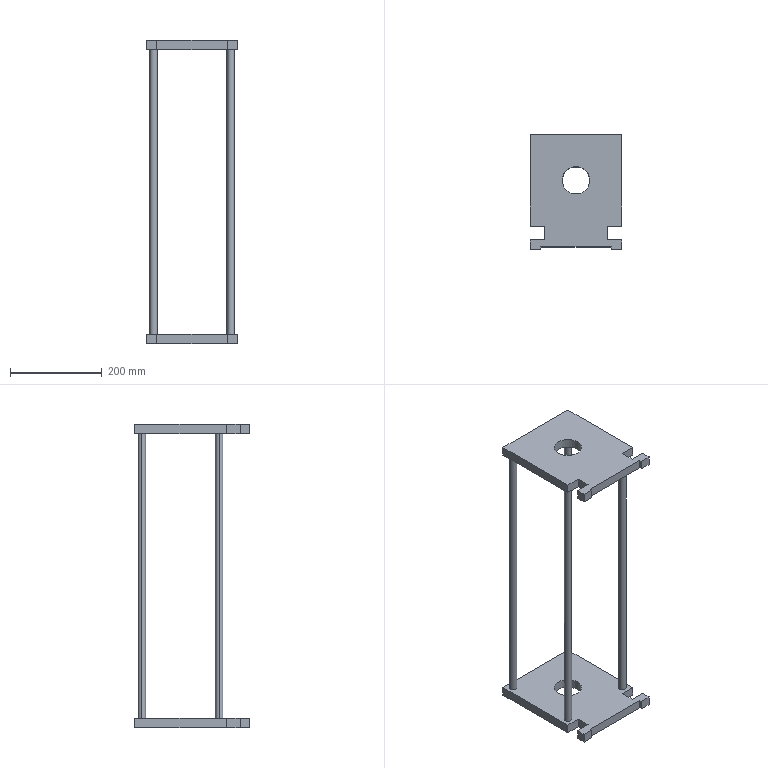Part | SolidWorks | features ICE 2, Extrusion 1 | 1 solid | 48 faces | box 200 x 250 x 660 mm | volume 2278181 mm3 | plane 36 | cylinder 12 | commonest cylinder face diameters 16 x8 60 x4
STEP:
#1=CARTESIAN_POINT('',(-30.,145.,660.));
#2=VERTEX_POINT('',#1);
#3=CARTESIAN_POINT('',(30.,145.,660.));
#4=VERTEX_POINT('',#3);
#5=CARTESIAN_POINT('',(0.,145.,660.));
#6=DIRECTION('',(0.,0.,1.));
#7=DIRECTION('',(1.,0.,0.));
#8=AXIS2_PLACEMENT_3D('',#5,#6,#7);
#9=CIRCLE('',#8,30.);
#10=EDGE_CURVE('',#2,#4,#9,.T.);
#11=ORIENTED_EDGE('',*,*,#10,.T.);
#12=CARTESIAN_POINT('',(30.,145.,640.));
#13=VERTEX_POINT('',#12);
#14=CARTESIAN_POINT('',(30.,145.,660.));
#15=DIRECTION('',(0.,0.,-1.));
#16=VECTOR('',#15,1000.);
#17=LINE('',#14,#16);
#18=EDGE_CURVE('',#4,#13,#17,.T.);
#19=ORIENTED_EDGE('',*,*,#18,.T.);
#20=CARTESIAN_POINT('',(-30.,145.,640.));
#21=VERTEX_POINT('',#20);
#22=CARTESIAN_POINT('',(0.,145.,640.));
#23=DIRECTION('',(0.,0.,1.));
#24=DIRECTION('',(1.,0.,0.));
#25=AXIS2_PLACEMENT_3D('',#22,#23,#24);
#26=CIRCLE('',#25,30.);
#27=EDGE_CURVE('',#21,#13,#26,.T.);
#28=ORIENTED_EDGE('',*,*,#27,.F.);
#29=CARTESIAN_POINT('',(-30.,145.,660.));
#30=DIRECTION('',(0.,0.,-1.));
#31=VECTOR('',#30,1000.);
#32=LINE('',#29,#31);
#33=EDGE_CURVE('',#2,#21,#32,.T.);
#34=ORIENTED_EDGE('',*,*,#33,.F.);
#35=EDGE_LOOP('',(#11,#19,#28,#34));
#36=FACE_OUTER_BOUND('',#35,.T.);
#37=CARTESIAN_POINT('',(0.,145.,660.));
#38=DIRECTION('',(0.,0.,-1.));
#39=DIRECTION('',(-1.,0.,0.));
#40=AXIS2_PLACEMENT_3D('',#37,#38,#39);
#41=CYLINDRICAL_SURFACE('',#40,30.);
#42=ADVANCED_FACE('',(#36),#41,.F.);
#43=CARTESIAN_POINT('',(-76.,61.,640.));
#44=VERTEX_POINT('',#43);
#45=CARTESIAN_POINT('',(-92.,61.,640.));
#46=VERTEX_POINT('',#45);
#47=CARTESIAN_POINT('',(-84.,61.,640.));
#48=DIRECTION('',(0.,0.,1.));
#49=DIRECTION('',(1.,0.,0.));
#50=AXIS2_PLACEMENT_3D('',#47,#48,#49);
#51=CIRCLE('',#50,8.);
#52=EDGE_CURVE('',#44,#46,#51,.T.);
#53=ORIENTED_EDGE('',*,*,#52,.F.);
#54=CARTESIAN_POINT('',(-76.,61.,20.));
#55=VERTEX_POINT('',#54);
#56=CARTESIAN_POINT('',(-76.,61.,640.));
#57=DIRECTION('',(0.,0.,-1.));
#58=VECTOR('',#57,1000.);
#59=LINE('',#56,#58);
#60=EDGE_CURVE('',#44,#55,#59,.T.);
#61=ORIENTED_EDGE('',*,*,#60,.T.);
#62=CARTESIAN_POINT('',(-92.,61.,20.));
#63=VERTEX_POINT('',#62);
#64=CARTESIAN_POINT('',(-84.,61.,20.));
#65=DIRECTION('',(0.,0.,1.));
#66=DIRECTION('',(-1.,0.,0.));
#67=AXIS2_PLACEMENT_3D('',#64,#65,#66);
#68=CIRCLE('',#67,8.);
#69=EDGE_CURVE('',#55,#63,#68,.T.);
#70=ORIENTED_EDGE('',*,*,#69,.T.);
#71=CARTESIAN_POINT('',(-92.,61.,640.));
#72=DIRECTION('',(0.,0.,-1.));
#73=VECTOR('',#72,1000.);
#74=LINE('',#71,#73);
#75=EDGE_CURVE('',#46,#63,#74,.T.);
#76=ORIENTED_EDGE('',*,*,#75,.F.);
#77=EDGE_LOOP('',(#53,#61,#70,#76));
#78=FACE_OUTER_BOUND('',#77,.T.);
#79=CARTESIAN_POINT('',(-84.,61.,640.));
#80=DIRECTION('',(0.,0.,-1.));
#81=DIRECTION('',(-1.,0.,0.));
#82=AXIS2_PLACEMENT_3D('',#79,#80,#81);
#83=CYLINDRICAL_SURFACE('',#82,8.);
#84=ADVANCED_FACE('',(#78),#83,.T.);
#85=CARTESIAN_POINT('',(92.,61.,640.));
#86=VERTEX_POINT('',#85);
#87=CARTESIAN_POINT('',(76.,61.,640.));
#88=VERTEX_POINT('',#87);
#89=CARTESIAN_POINT('',(84.,61.,640.));
#90=DIRECTION('',(0.,0.,1.));
#91=DIRECTION('',(1.,0.,0.));
#92=AXIS2_PLACEMENT_3D('',#89,#90,#91);
#93=CIRCLE('',#92,8.);
#94=EDGE_CURVE('',#86,#88,#93,.T.);
#95=ORIENTED_EDGE('',*,*,#94,.F.);
#96=CARTESIAN_POINT('',(92.,61.,20.));
#97=VERTEX_POINT('',#96);
#98=CARTESIAN_POINT('',(92.,61.,640.));
#99=DIRECTION('',(0.,0.,-1.));
#100=VECTOR('',#99,1000.);
#101=LINE('',#98,#100);
#102=EDGE_CURVE('',#86,#97,#101,.T.);
#103=ORIENTED_EDGE('',*,*,#102,.T.);
#104=CARTESIAN_POINT('',(76.,61.,20.));
#105=VERTEX_POINT('',#104);
#106=CARTESIAN_POINT('',(84.,61.,20.));
#107=DIRECTION('',(0.,0.,1.));
#108=DIRECTION('',(-1.,0.,0.));
#109=AXIS2_PLACEMENT_3D('',#106,#107,#108);
#110=CIRCLE('',#109,8.);
#111=EDGE_CURVE('',#97,#105,#110,.T.);
#112=ORIENTED_EDGE('',*,*,#111,.T.);
#113=CARTESIAN_POINT('',(76.,61.,640.));
#114=DIRECTION('',(0.,0.,-1.));
#115=VECTOR('',#114,1000.);
#116=LINE('',#113,#115);
#117=EDGE_CURVE('',#88,#105,#116,.T.);
#118=ORIENTED_EDGE('',*,*,#117,.F.);
#119=EDGE_LOOP('',(#95,#103,#112,#118));
#120=FACE_OUTER_BOUND('',#119,.T.);
#121=CARTESIAN_POINT('',(84.,61.,640.));
#122=DIRECTION('',(0.,0.,-1.));
#123=DIRECTION('',(-1.,0.,0.));
#124=AXIS2_PLACEMENT_3D('',#121,#122,#123);
#125=CYLINDRICAL_SURFACE('',#124,8.);
#126=ADVANCED_FACE('',(#120),#125,.T.);
#127=CARTESIAN_POINT('',(92.,229.,640.));
#128=VERTEX_POINT('',#127);
#129=CARTESIAN_POINT('',(76.,229.,640.));
#130=VERTEX_POINT('',#129);
#131=CARTESIAN_POINT('',(84.,229.,640.));
#132=DIRECTION('',(0.,0.,1.));
#133=DIRECTION('',(1.,0.,0.));
#134=AXIS2_PLACEMENT_3D('',#131,#132,#133);
#135=CIRCLE('',#134,8.);
#136=EDGE_CURVE('',#128,#130,#135,.T.);
#137=ORIENTED_EDGE('',*,*,#136,.F.);
#138=CARTESIAN_POINT('',(92.,229.,20.));
#139=VERTEX_POINT('',#138);
#140=CARTESIAN_POINT('',(92.,229.,640.));
#141=DIRECTION('',(0.,0.,-1.));
#142=VECTOR('',#141,1000.);
#143=LINE('',#140,#142);
#144=EDGE_CURVE('',#128,#139,#143,.T.);
#145=ORIENTED_EDGE('',*,*,#144,.T.);
#146=CARTESIAN_POINT('',(76.,229.,20.));
#147=VERTEX_POINT('',#146);
#148=CARTESIAN_POINT('',(84.,229.,20.));
#149=DIRECTION('',(0.,0.,1.));
#150=DIRECTION('',(-1.,0.,0.));
#151=AXIS2_PLACEMENT_3D('',#148,#149,#150);
#152=CIRCLE('',#151,8.);
#153=EDGE_CURVE('',#139,#147,#152,.T.);
#154=ORIENTED_EDGE('',*,*,#153,.T.);
#155=CARTESIAN_POINT('',(76.,229.,640.));
#156=DIRECTION('',(0.,0.,-1.));
#157=VECTOR('',#156,1000.);
#158=LINE('',#155,#157);
#159=EDGE_CURVE('',#130,#147,#158,.T.);
#160=ORIENTED_EDGE('',*,*,#159,.F.);
#161=EDGE_LOOP('',(#137,#145,#154,#160));
#162=FACE_OUTER_BOUND('',#161,.T.);
#163=CARTESIAN_POINT('',(84.,229.,640.));
#164=DIRECTION('',(0.,0.,-1.));
#165=DIRECTION('',(-1.,0.,0.));
#166=AXIS2_PLACEMENT_3D('',#163,#164,#165);
#167=CYLINDRICAL_SURFACE('',#166,8.);
#168=ADVANCED_FACE('',(#162),#167,.T.);
#169=CARTESIAN_POINT('',(-76.,229.,640.));
#170=VERTEX_POINT('',#169);
#171=CARTESIAN_POINT('',(-92.,229.,640.));
#172=VERTEX_POINT('',#171);
#173=CARTESIAN_POINT('',(-84.,229.,640.));
#174=DIRECTION('',(0.,0.,1.));
#175=DIRECTION('',(1.,0.,0.));
#176=AXIS2_PLACEMENT_3D('',#173,#174,#175);
#177=CIRCLE('',#176,8.);
#178=EDGE_CURVE('',#170,#172,#177,.T.);
#179=ORIENTED_EDGE('',*,*,#178,.F.);
#180=CARTESIAN_POINT('',(-76.,229.,20.));
#181=VERTEX_POINT('',#180);
#182=CARTESIAN_POINT('',(-76.,229.,640.));
#183=DIRECTION('',(0.,0.,-1.));
#184=VECTOR('',#183,1000.);
#185=LINE('',#182,#184);
#186=EDGE_CURVE('',#170,#181,#185,.T.);
#187=ORIENTED_EDGE('',*,*,#186,.T.);
#188=CARTESIAN_POINT('',(-92.,229.,20.));
#189=VERTEX_POINT('',#188);
#190=CARTESIAN_POINT('',(-84.,229.,20.));
#191=DIRECTION('',(0.,0.,1.));
#192=DIRECTION('',(-1.,0.,0.));
#193=AXIS2_PLACEMENT_3D('',#190,#191,#192);
#194=CIRCLE('',#193,8.);
#195=EDGE_CURVE('',#181,#189,#194,.T.);
#196=ORIENTED_EDGE('',*,*,#195,.T.);
#197=CARTESIAN_POINT('',(-92.,229.,640.));
#198=DIRECTION('',(0.,0.,-1.));
#199=VECTOR('',#198,1000.);
#200=LINE('',#197,#199);
#201=EDGE_CURVE('',#172,#189,#200,.T.);
#202=ORIENTED_EDGE('',*,*,#201,.F.);
#203=EDGE_LOOP('',(#179,#187,#196,#202));
#204=FACE_OUTER_BOUND('',#203,.T.);
#205=CARTESIAN_POINT('',(-84.,229.,640.));
#206=DIRECTION('',(0.,0.,-1.));
#207=DIRECTION('',(-1.,0.,0.));
#208=AXIS2_PLACEMENT_3D('',#205,#206,#207);
#209=CYLINDRICAL_SURFACE('',#208,8.);
#210=ADVANCED_FACE('',(#204),#209,.T.);
#211=CARTESIAN_POINT('',(-30.,145.,20.));
#212=VERTEX_POINT('',#211);
#213=CARTESIAN_POINT('',(30.,145.,20.));
#214=VERTEX_POINT('',#213);
#215=CARTESIAN_POINT('',(0.,145.,20.));
#216=DIRECTION('',(0.,0.,1.));
#217=DIRECTION('',(1.,0.,0.));
#218=AXIS2_PLACEMENT_3D('',#215,#216,#217);
#219=CIRCLE('',#218,30.);
#220=EDGE_CURVE('',#212,#214,#219,.T.);
#221=ORIENTED_EDGE('',*,*,#220,.T.);
#222=CARTESIAN_POINT('',(30.,145.,0.));
#223=VERTEX_POINT('',#222);
#224=CARTESIAN_POINT('',(30.,145.,20.));
#225=DIRECTION('',(0.,0.,-1.));
#226=VECTOR('',#225,1000.);
#227=LINE('',#224,#226);
#228=EDGE_CURVE('',#214,#223,#227,.T.);
#229=ORIENTED_EDGE('',*,*,#228,.T.);
#230=CARTESIAN_POINT('',(-30.,145.,0.));
#231=VERTEX_POINT('',#230);
#232=CARTESIAN_POINT('',(0.,145.,0.));
#233=DIRECTION('',(0.,0.,1.));
#234=DIRECTION('',(1.,0.,0.));
#235=AXIS2_PLACEMENT_3D('',#232,#233,#234);
#236=CIRCLE('',#235,30.);
#237=EDGE_CURVE('',#231,#223,#236,.T.);
#238=ORIENTED_EDGE('',*,*,#237,.F.);
#239=CARTESIAN_POINT('',(-30.,145.,20.));
#240=DIRECTION('',(0.,0.,-1.));
#241=VECTOR('',#240,1000.);
#242=LINE('',#239,#241);
#243=EDGE_CURVE('',#212,#231,#242,.T.);
#244=ORIENTED_EDGE('',*,*,#243,.F.);
#245=EDGE_LOOP('',(#221,#229,#238,#244));
#246=FACE_OUTER_BOUND('',#245,.T.);
#247=CARTESIAN_POINT('',(0.,145.,20.));
#248=DIRECTION('',(0.,0.,-1.));
#249=DIRECTION('',(-1.,0.,0.));
#250=AXIS2_PLACEMENT_3D('',#247,#248,#249);
#251=CYLINDRICAL_SURFACE('',#250,30.);
#252=ADVANCED_FACE('',(#246),#251,.F.);
#253=CARTESIAN_POINT('',(-84.,61.,20.));
#254=DIRECTION('',(0.,0.,1.));
#255=DIRECTION('',(-1.,0.,0.));
#256=AXIS2_PLACEMENT_3D('',#253,#254,#255);
#257=CIRCLE('',#256,8.);
#258=EDGE_CURVE('',#63,#55,#257,.T.);
#259=ORIENTED_EDGE('',*,*,#258,.F.);
#260=ORIENTED_EDGE('',*,*,#69,.F.);
#261=EDGE_LOOP('',(#259,#260));
#262=FACE_BOUND('',#261,.T.);
#263=CARTESIAN_POINT('',(84.,61.,20.));
#264=DIRECTION('',(0.,0.,1.));
#265=DIRECTION('',(-1.,0.,0.));
#266=AXIS2_PLACEMENT_3D('',#263,#264,#265);
#267=CIRCLE('',#266,8.);
#268=EDGE_CURVE('',#105,#97,#267,.T.);
#269=ORIENTED_EDGE('',*,*,#268,.F.);
#270=ORIENTED_EDGE('',*,*,#111,.F.);
#271=EDGE_LOOP('',(#269,#270));
#272=FACE_BOUND('',#271,.T.);
#273=CARTESIAN_POINT('',(84.,229.,20.));
#274=DIRECTION('',(0.,0.,1.));
#275=DIRECTION('',(-1.,0.,0.));
#276=AXIS2_PLACEMENT_3D('',#273,#274,#275);
#277=CIRCLE('',#276,8.);
#278=EDGE_CURVE('',#147,#139,#277,.T.);
#279=ORIENTED_EDGE('',*,*,#278,.F.);
#280=ORIENTED_EDGE('',*,*,#153,.F.);
#281=EDGE_LOOP('',(#279,#280));
#282=FACE_BOUND('',#281,.T.);
#283=CARTESIAN_POINT('',(-84.,229.,20.));
#284=DIRECTION('',(0.,0.,1.));
#285=DIRECTION('',(-1.,0.,0.));
#286=AXIS2_PLACEMENT_3D('',#283,#284,#285);
#287=CIRCLE('',#286,8.);
#288=EDGE_CURVE('',#189,#181,#287,.T.);
#289=ORIENTED_EDGE('',*,*,#288,.F.);
#290=ORIENTED_EDGE('',*,*,#195,.F.);
#291=EDGE_LOOP('',(#289,#290));
#292=FACE_BOUND('',#291,.T.);
#293=CARTESIAN_POINT('',(-76.389,-5.,20.));
#294=VERTEX_POINT('',#293);
#295=CARTESIAN_POINT('',(-76.389,0.,20.));
#296=VERTEX_POINT('',#295);
#297=CARTESIAN_POINT('',(-76.389,0.,20.));
#298=DIRECTION('',(0.,1.,0.));
#299=VECTOR('',#298,1000.);
#300=LINE('',#297,#299);
#301=EDGE_CURVE('',#294,#296,#300,.T.);
#302=ORIENTED_EDGE('',*,*,#301,.T.);
#303=CARTESIAN_POINT('',(76.389,0.,20.));
#304=VERTEX_POINT('',#303);
#305=CARTESIAN_POINT('',(76.389,0.,20.));
#306=DIRECTION('',(1.,0.,0.));
#307=VECTOR('',#306,1000.);
#308=LINE('',#305,#307);
#309=EDGE_CURVE('',#296,#304,#308,.T.);
#310=ORIENTED_EDGE('',*,*,#309,.T.);
#311=CARTESIAN_POINT('',(76.389,-5.,20.));
#312=VERTEX_POINT('',#311);
#313=CARTESIAN_POINT('',(76.389,0.,20.));
#314=DIRECTION('',(0.,-1.,0.));
#315=VECTOR('',#314,1000.);
#316=LINE('',#313,#315);
#317=EDGE_CURVE('',#304,#312,#316,.T.);
#318=ORIENTED_EDGE('',*,*,#317,.T.);
#319=CARTESIAN_POINT('',(100.,-5.,20.));
#320=VERTEX_POINT('',#319);
#321=CARTESIAN_POINT('',(76.389,-5.,20.));
#322=DIRECTION('',(1.,0.,0.));
#323=VECTOR('',#322,1000.);
#324=LINE('',#321,#323);
#325=EDGE_CURVE('',#312,#320,#324,.T.);
#326=ORIENTED_EDGE('',*,*,#325,.T.);
#327=CARTESIAN_POINT('',(100.,15.,20.));
#328=VERTEX_POINT('',#327);
#329=CARTESIAN_POINT('',(100.,-5.,20.));
#330=DIRECTION('',(0.,1.,0.));
#331=VECTOR('',#330,1000.);
#332=LINE('',#329,#331);
#333=EDGE_CURVE('',#320,#328,#332,.T.);
#334=ORIENTED_EDGE('',*,*,#333,.T.);
#335=CARTESIAN_POINT('',(68.,15.,20.));
#336=VERTEX_POINT('',#335);
#337=CARTESIAN_POINT('',(100.,15.,20.));
#338=DIRECTION('',(-1.,0.,0.));
#339=VECTOR('',#338,1000.);
#340=LINE('',#337,#339);
#341=EDGE_CURVE('',#328,#336,#340,.T.);
#342=ORIENTED_EDGE('',*,*,#341,.T.);
#343=CARTESIAN_POINT('',(68.,45.,20.));
#344=VERTEX_POINT('',#343);
#345=CARTESIAN_POINT('',(68.,15.,20.));
#346=DIRECTION('',(0.,1.,0.));
#347=VECTOR('',#346,1000.);
#348=LINE('',#345,#347);
#349=EDGE_CURVE('',#336,#344,#348,.T.);
#350=ORIENTED_EDGE('',*,*,#349,.T.);
#351=CARTESIAN_POINT('',(100.,45.,20.));
#352=VERTEX_POINT('',#351);
#353=CARTESIAN_POINT('',(68.,45.,20.));
#354=DIRECTION('',(1.,0.,0.));
#355=VECTOR('',#354,1000.);
#356=LINE('',#353,#355);
#357=EDGE_CURVE('',#344,#352,#356,.T.);
#358=ORIENTED_EDGE('',*,*,#357,.T.);
#359=CARTESIAN_POINT('',(100.,245.,20.));
#360=VERTEX_POINT('',#359);
#361=CARTESIAN_POINT('',(100.,45.,20.));
#362=DIRECTION('',(0.,1.,0.));
#363=VECTOR('',#362,1000.);
#364=LINE('',#361,#363);
#365=EDGE_CURVE('',#352,#360,#364,.T.);
#366=ORIENTED_EDGE('',*,*,#365,.T.);
#367=CARTESIAN_POINT('',(-100.,245.,20.));
#368=VERTEX_POINT('',#367);
#369=CARTESIAN_POINT('',(-100.,245.,20.));
#370=DIRECTION('',(-1.,0.,0.));
#371=VECTOR('',#370,1000.);
#372=LINE('',#369,#371);
#373=EDGE_CURVE('',#360,#368,#372,.T.);
#374=ORIENTED_EDGE('',*,*,#373,.T.);
#375=CARTESIAN_POINT('',(-100.,45.,20.));
#376=VERTEX_POINT('',#375);
#377=CARTESIAN_POINT('',(-100.,45.,20.));
#378=DIRECTION('',(0.,-1.,0.));
#379=VECTOR('',#378,1000.);
#380=LINE('',#377,#379);
#381=EDGE_CURVE('',#368,#376,#380,.T.);
#382=ORIENTED_EDGE('',*,*,#381,.T.);
#383=CARTESIAN_POINT('',(-68.,45.,20.));
#384=VERTEX_POINT('',#383);
#385=CARTESIAN_POINT('',(-68.,45.,20.));
#386=DIRECTION('',(1.,0.,0.));
#387=VECTOR('',#386,1000.);
#388=LINE('',#385,#387);
#389=EDGE_CURVE('',#376,#384,#388,.T.);
#390=ORIENTED_EDGE('',*,*,#389,.T.);
#391=CARTESIAN_POINT('',(-68.,15.,20.));
#392=VERTEX_POINT('',#391);
#393=CARTESIAN_POINT('',(-68.,15.,20.));
#394=DIRECTION('',(0.,-1.,0.));
#395=VECTOR('',#394,1000.);
#396=LINE('',#393,#395);
#397=EDGE_CURVE('',#384,#392,#396,.T.);
#398=ORIENTED_EDGE('',*,*,#397,.T.);
#399=CARTESIAN_POINT('',(-100.,15.,20.));
#400=VERTEX_POINT('',#399);
#401=CARTESIAN_POINT('',(-100.,15.,20.));
#402=DIRECTION('',(-1.,0.,0.));
#403=VECTOR('',#402,1000.);
#404=LINE('',#401,#403);
#405=EDGE_CURVE('',#392,#400,#404,.T.);
#406=ORIENTED_EDGE('',*,*,#405,.T.);
#407=CARTESIAN_POINT('',(-100.,-5.,20.));
#408=VERTEX_POINT('',#407);
#409=CARTESIAN_POINT('',(-100.,-5.,20.));
#410=DIRECTION('',(0.,-1.,0.));
#411=VECTOR('',#410,1000.);
#412=LINE('',#409,#411);
#413=EDGE_CURVE('',#400,#408,#412,.T.);
#414=ORIENTED_EDGE('',*,*,#413,.T.);
#415=CARTESIAN_POINT('',(-76.389,-5.,20.));
#416=DIRECTION('',(1.,0.,0.));
#417=VECTOR('',#416,1000.);
#418=LINE('',#415,#417);
#419=EDGE_CURVE('',#408,#294,#418,.T.);
#420=ORIENTED_EDGE('',*,*,#419,.T.);
#421=EDGE_LOOP('',(#302,#310,#318,#326,#334,#342,#350,#358,#366,#374,#382,#390,#398,#406,#414,#420));
#422=FACE_OUTER_BOUND('',#421,.T.);
#423=ORIENTED_EDGE('',*,*,#220,.F.);
#424=CARTESIAN_POINT('',(0.,145.,20.));
#425=DIRECTION('',(0.,0.,1.));
#426=DIRECTION('',(1.,0.,0.));
#427=AXIS2_PLACEMENT_3D('',#424,#425,#426);
#428=CIRCLE('',#427,30.);
#429=EDGE_CURVE('',#214,#212,#428,.T.);
#430=ORIENTED_EDGE('',*,*,#429,.F.);
#431=EDGE_LOOP('',(#423,#430));
#432=FACE_BOUND('',#431,.T.);
#433=CARTESIAN_POINT('',(0.,0.,20.));
#434=DIRECTION('',(0.,0.,-1.));
#435=DIRECTION('',(-1.,0.,0.));
#436=AXIS2_PLACEMENT_3D('',#433,#434,#435);
#437=PLANE('',#436);
#438=ADVANCED_FACE('',(#262,#272,#282,#292,#422,#432),#437,.F.);
#439=CARTESIAN_POINT('',(-76.389,-5.,0.));
#440=VERTEX_POINT('',#439);
#441=CARTESIAN_POINT('',(-76.389,0.,0.));
#442=VERTEX_POINT('',#441);
#443=CARTESIAN_POINT('',(-76.389,0.,0.));
#444=DIRECTION('',(0.,1.,0.));
#445=VECTOR('',#444,1000.);
#446=LINE('',#443,#445);
#447=EDGE_CURVE('',#440,#442,#446,.T.);
#448=ORIENTED_EDGE('',*,*,#447,.F.);
#449=CARTESIAN_POINT('',(-100.,-5.,0.));
#450=VERTEX_POINT('',#449);
#451=CARTESIAN_POINT('',(-76.389,-5.,0.));
#452=DIRECTION('',(1.,0.,0.));
#453=VECTOR('',#452,1000.);
#454=LINE('',#451,#453);
#455=EDGE_CURVE('',#450,#440,#454,.T.);
#456=ORIENTED_EDGE('',*,*,#455,.F.);
#457=CARTESIAN_POINT('',(-100.,15.,0.));
#458=VERTEX_POINT('',#457);
#459=CARTESIAN_POINT('',(-100.,-5.,0.));
#460=DIRECTION('',(0.,-1.,0.));
#461=VECTOR('',#460,1000.);
#462=LINE('',#459,#461);
#463=EDGE_CURVE('',#458,#450,#462,.T.);
#464=ORIENTED_EDGE('',*,*,#463,.F.);
#465=CARTESIAN_POINT('',(-68.,15.,0.));
#466=VERTEX_POINT('',#465);
#467=CARTESIAN_POINT('',(-100.,15.,0.));
#468=DIRECTION('',(-1.,0.,0.));
#469=VECTOR('',#468,1000.);
#470=LINE('',#467,#469);
#471=EDGE_CURVE('',#466,#458,#470,.T.);
#472=ORIENTED_EDGE('',*,*,#471,.F.);
#473=CARTESIAN_POINT('',(-68.,45.,0.));
#474=VERTEX_POINT('',#473);
#475=CARTESIAN_POINT('',(-68.,15.,0.));
#476=DIRECTION('',(0.,-1.,0.));
#477=VECTOR('',#476,1000.);
#478=LINE('',#475,#477);
#479=EDGE_CURVE('',#474,#466,#478,.T.);
#480=ORIENTED_EDGE('',*,*,#479,.F.);
#481=CARTESIAN_POINT('',(-100.,45.,0.));
#482=VERTEX_POINT('',#481);
#483=CARTESIAN_POINT('',(-68.,45.,0.));
#484=DIRECTION('',(1.,0.,0.));
#485=VECTOR('',#484,1000.);
#486=LINE('',#483,#485);
#487=EDGE_CURVE('',#482,#474,#486,.T.);
#488=ORIENTED_EDGE('',*,*,#487,.F.);
#489=CARTESIAN_POINT('',(-100.,245.,0.));
#490=VERTEX_POINT('',#489);
#491=CARTESIAN_POINT('',(-100.,45.,0.));
#492=DIRECTION('',(0.,-1.,0.));
#493=VECTOR('',#492,1000.);
#494=LINE('',#491,#493);
#495=EDGE_CURVE('',#490,#482,#494,.T.);
#496=ORIENTED_EDGE('',*,*,#495,.F.);
#497=CARTESIAN_POINT('',(100.,245.,0.));
#498=VERTEX_POINT('',#497);
#499=CARTESIAN_POINT('',(-100.,245.,0.));
#500=DIRECTION('',(-1.,0.,0.));
#501=VECTOR('',#500,1000.);
#502=LINE('',#499,#501);
#503=EDGE_CURVE('',#498,#490,#502,.T.);
#504=ORIENTED_EDGE('',*,*,#503,.F.);
#505=CARTESIAN_POINT('',(100.,45.,0.));
#506=VERTEX_POINT('',#505);
#507=CARTESIAN_POINT('',(100.,45.,0.));
#508=DIRECTION('',(0.,1.,0.));
#509=VECTOR('',#508,1000.);
#510=LINE('',#507,#509);
#511=EDGE_CURVE('',#506,#498,#510,.T.);
#512=ORIENTED_EDGE('',*,*,#511,.F.);
#513=CARTESIAN_POINT('',(68.,45.,0.));
#514=VERTEX_POINT('',#513);
#515=CARTESIAN_POINT('',(68.,45.,0.));
#516=DIRECTION('',(1.,0.,0.));
#517=VECTOR('',#516,1000.);
#518=LINE('',#515,#517);
#519=EDGE_CURVE('',#514,#506,#518,.T.);
#520=ORIENTED_EDGE('',*,*,#519,.F.);
#521=CARTESIAN_POINT('',(68.,15.,0.));
#522=VERTEX_POINT('',#521);
#523=CARTESIAN_POINT('',(68.,15.,0.));
#524=DIRECTION('',(0.,1.,0.));
#525=VECTOR('',#524,1000.);
#526=LINE('',#523,#525);
#527=EDGE_CURVE('',#522,#514,#526,.T.);
#528=ORIENTED_EDGE('',*,*,#527,.F.);
#529=CARTESIAN_POINT('',(100.,15.,0.));
#530=VERTEX_POINT('',#529);
#531=CARTESIAN_POINT('',(100.,15.,0.));
#532=DIRECTION('',(-1.,0.,0.));
#533=VECTOR('',#532,1000.);
#534=LINE('',#531,#533);
#535=EDGE_CURVE('',#530,#522,#534,.T.);
#536=ORIENTED_EDGE('',*,*,#535,.F.);
#537=CARTESIAN_POINT('',(100.,-5.,0.));
#538=VERTEX_POINT('',#537);
#539=CARTESIAN_POINT('',(100.,-5.,0.));
#540=DIRECTION('',(0.,1.,0.));
#541=VECTOR('',#540,1000.);
#542=LINE('',#539,#541);
#543=EDGE_CURVE('',#538,#530,#542,.T.);
#544=ORIENTED_EDGE('',*,*,#543,.F.);
#545=CARTESIAN_POINT('',(76.389,-5.,0.));
#546=VERTEX_POINT('',#545);
#547=CARTESIAN_POINT('',(76.389,-5.,0.));
#548=DIRECTION('',(1.,0.,0.));
#549=VECTOR('',#548,1000.);
#550=LINE('',#547,#549);
#551=EDGE_CURVE('',#546,#538,#550,.T.);
#552=ORIENTED_EDGE('',*,*,#551,.F.);
#553=CARTESIAN_POINT('',(76.389,0.,0.));
#554=VERTEX_POINT('',#553);
#555=CARTESIAN_POINT('',(76.389,0.,0.));
#556=DIRECTION('',(0.,-1.,0.));
#557=VECTOR('',#556,1000.);
#558=LINE('',#555,#557);
#559=EDGE_CURVE('',#554,#546,#558,.T.);
#560=ORIENTED_EDGE('',*,*,#559,.F.);
#561=CARTESIAN_POINT('',(76.389,0.,0.));
#562=DIRECTION('',(1.,0.,0.));
#563=VECTOR('',#562,1000.);
#564=LINE('',#561,#563);
#565=EDGE_CURVE('',#442,#554,#564,.T.);
#566=ORIENTED_EDGE('',*,*,#565,.F.);
#567=EDGE_LOOP('',(#448,#456,#464,#472,#480,#488,#496,#504,#512,#520,#528,#536,#544,#552,#560,#566));
#568=FACE_OUTER_BOUND('',#567,.T.);
#569=ORIENTED_EDGE('',*,*,#237,.T.);
#570=CARTESIAN_POINT('',(0.,145.,0.));
#571=DIRECTION('',(0.,0.,1.));
#572=DIRECTION('',(1.,0.,0.));
#573=AXIS2_PLACEMENT_3D('',#570,#571,#572);
#574=CIRCLE('',#573,30.);
#575=EDGE_CURVE('',#223,#231,#574,.T.);
#576=ORIENTED_EDGE('',*,*,#575,.T.);
#577=EDGE_LOOP('',(#569,#576));
#578=FACE_BOUND('',#577,.T.);
#579=CARTESIAN_POINT('',(0.,0.,0.));
#580=DIRECTION('',(0.,0.,-1.));
#581=DIRECTION('',(-1.,0.,0.));
#582=AXIS2_PLACEMENT_3D('',#579,#580,#581);
#583=PLANE('',#582);
#584=ADVANCED_FACE('',(#568,#578),#583,.T.);
#585=ORIENTED_EDGE('',*,*,#447,.T.);
#586=CARTESIAN_POINT('',(-76.389,0.,20.));
#587=DIRECTION('',(0.,0.,-1.));
#588=VECTOR('',#587,1000.);
#589=LINE('',#586,#588);
#590=EDGE_CURVE('',#296,#442,#589,.T.);
#591=ORIENTED_EDGE('',*,*,#590,.F.);
#592=ORIENTED_EDGE('',*,*,#301,.F.);
#593=CARTESIAN_POINT('',(-76.389,-5.,20.));
#594=DIRECTION('',(0.,0.,-1.));
#595=VECTOR('',#594,1000.);
#596=LINE('',#593,#595);
#597=EDGE_CURVE('',#294,#440,#596,.T.);
#598=ORIENTED_EDGE('',*,*,#597,.T.);
#599=EDGE_LOOP('',(#585,#591,#592,#598));
#600=FACE_OUTER_BOUND('',#599,.T.);
#601=CARTESIAN_POINT('',(-76.389,0.,20.));
#602=DIRECTION('',(-1.,0.,0.));
#603=DIRECTION('',(0.,0.,1.));
#604=AXIS2_PLACEMENT_3D('',#601,#602,#603);
#605=PLANE('',#604);
#606=ADVANCED_FACE('',(#600),#605,.F.);
#607=ORIENTED_EDGE('',*,*,#565,.T.);
#608=CARTESIAN_POINT('',(76.389,0.,20.));
#609=DIRECTION('',(0.,0.,-1.));
#610=VECTOR('',#609,1000.);
#611=LINE('',#608,#610);
#612=EDGE_CURVE('',#304,#554,#611,.T.);
#613=ORIENTED_EDGE('',*,*,#612,.F.);
#614=ORIENTED_EDGE('',*,*,#309,.F.);
#615=ORIENTED_EDGE('',*,*,#590,.T.);
#616=EDGE_LOOP('',(#607,#613,#614,#615));
#617=FACE_OUTER_BOUND('',#616,.T.);
#618=CARTESIAN_POINT('',(76.389,0.,20.));
#619=DIRECTION('',(0.,1.,0.));
#620=DIRECTION('',(-1.,0.,0.));
#621=AXIS2_PLACEMENT_3D('',#618,#619,#620);
#622=PLANE('',#621);
#623=ADVANCED_FACE('',(#617),#622,.F.);
#624=ORIENTED_EDGE('',*,*,#559,.T.);
#625=CARTESIAN_POINT('',(76.389,-5.,20.));
#626=DIRECTION('',(0.,0.,-1.));
#627=VECTOR('',#626,1000.);
#628=LINE('',#625,#627);
#629=EDGE_CURVE('',#312,#546,#628,.T.);
#630=ORIENTED_EDGE('',*,*,#629,.F.);
#631=ORIENTED_EDGE('',*,*,#317,.F.);
#632=ORIENTED_EDGE('',*,*,#612,.T.);
#633=EDGE_LOOP('',(#624,#630,#631,#632));
#634=FACE_OUTER_BOUND('',#633,.T.);
#635=CARTESIAN_POINT('',(76.389,0.,20.));
#636=DIRECTION('',(1.,0.,0.));
#637=DIRECTION('',(0.,0.,-1.));
#638=AXIS2_PLACEMENT_3D('',#635,#636,#637);
#639=PLANE('',#638);
#640=ADVANCED_FACE('',(#634),#639,.F.);
#641=ORIENTED_EDGE('',*,*,#551,.T.);
#642=CARTESIAN_POINT('',(100.,-5.,20.));
#643=DIRECTION('',(0.,0.,-1.));
#644=VECTOR('',#643,1000.);
#645=LINE('',#642,#644);
#646=EDGE_CURVE('',#320,#538,#645,.T.);
#647=ORIENTED_EDGE('',*,*,#646,.F.);
#648=ORIENTED_EDGE('',*,*,#325,.F.);
#649=ORIENTED_EDGE('',*,*,#629,.T.);
#650=EDGE_LOOP('',(#641,#647,#648,#649));
#651=FACE_OUTER_BOUND('',#650,.T.);
#652=CARTESIAN_POINT('',(76.389,-5.,20.));
#653=DIRECTION('',(0.,1.,0.));
#654=DIRECTION('',(-1.,0.,0.));
#655=AXIS2_PLACEMENT_3D('',#652,#653,#654);
#656=PLANE('',#655);
#657=ADVANCED_FACE('',(#651),#656,.F.);
#658=ORIENTED_EDGE('',*,*,#543,.T.);
#659=CARTESIAN_POINT('',(100.,15.,20.));
#660=DIRECTION('',(0.,0.,-1.));
#661=VECTOR('',#660,1000.);
#662=LINE('',#659,#661);
#663=EDGE_CURVE('',#328,#530,#662,.T.);
#664=ORIENTED_EDGE('',*,*,#663,.F.);
#665=ORIENTED_EDGE('',*,*,#333,.F.);
#666=ORIENTED_EDGE('',*,*,#646,.T.);
#667=EDGE_LOOP('',(#658,#664,#665,#666));
#668=FACE_OUTER_BOUND('',#667,.T.);
#669=CARTESIAN_POINT('',(100.,-5.,20.));
#670=DIRECTION('',(-1.,0.,0.));
#671=DIRECTION('',(0.,0.,1.));
#672=AXIS2_PLACEMENT_3D('',#669,#670,#671);
#673=PLANE('',#672);
#674=ADVANCED_FACE('',(#668),#673,.F.);
#675=ORIENTED_EDGE('',*,*,#535,.T.);
#676=CARTESIAN_POINT('',(68.,15.,20.));
#677=DIRECTION('',(0.,0.,-1.));
#678=VECTOR('',#677,1000.);
#679=LINE('',#676,#678);
#680=EDGE_CURVE('',#336,#522,#679,.T.);
#681=ORIENTED_EDGE('',*,*,#680,.F.);
#682=ORIENTED_EDGE('',*,*,#341,.F.);
#683=ORIENTED_EDGE('',*,*,#663,.T.);
#684=EDGE_LOOP('',(#675,#681,#682,#683));
#685=FACE_OUTER_BOUND('',#684,.T.);
#686=CARTESIAN_POINT('',(100.,15.,20.));
#687=DIRECTION('',(0.,-1.,0.));
#688=DIRECTION('',(1.,0.,0.));
#689=AXIS2_PLACEMENT_3D('',#686,#687,#688);
#690=PLANE('',#689);
#691=ADVANCED_FACE('',(#685),#690,.F.);
#692=ORIENTED_EDGE('',*,*,#527,.T.);
#693=CARTESIAN_POINT('',(68.,45.,20.));
#694=DIRECTION('',(0.,0.,-1.));
#695=VECTOR('',#694,1000.);
#696=LINE('',#693,#695);
#697=EDGE_CURVE('',#344,#514,#696,.T.);
#698=ORIENTED_EDGE('',*,*,#697,.F.);
#699=ORIENTED_EDGE('',*,*,#349,.F.);
#700=ORIENTED_EDGE('',*,*,#680,.T.);
#701=EDGE_LOOP('',(#692,#698,#699,#700));
#702=FACE_OUTER_BOUND('',#701,.T.);
#703=CARTESIAN_POINT('',(68.,15.,20.));
#704=DIRECTION('',(-1.,0.,0.));
#705=DIRECTION('',(0.,0.,1.));
#706=AXIS2_PLACEMENT_3D('',#703,#704,#705);
#707=PLANE('',#706);
#708=ADVANCED_FACE('',(#702),#707,.F.);
#709=ORIENTED_EDGE('',*,*,#519,.T.);
#710=CARTESIAN_POINT('',(100.,45.,20.));
#711=DIRECTION('',(0.,0.,-1.));
#712=VECTOR('',#711,1000.);
#713=LINE('',#710,#712);
#714=EDGE_CURVE('',#352,#506,#713,.T.);
#715=ORIENTED_EDGE('',*,*,#714,.F.);
#716=ORIENTED_EDGE('',*,*,#357,.F.);
#717=ORIENTED_EDGE('',*,*,#697,.T.);
#718=EDGE_LOOP('',(#709,#715,#716,#717));
#719=FACE_OUTER_BOUND('',#718,.T.);
#720=CARTESIAN_POINT('',(68.,45.,20.));
#721=DIRECTION('',(0.,1.,0.));
#722=DIRECTION('',(0.,0.,1.));
#723=AXIS2_PLACEMENT_3D('',#720,#721,#722);
#724=PLANE('',#723);
#725=ADVANCED_FACE('',(#719),#724,.F.);
#726=ORIENTED_EDGE('',*,*,#511,.T.);
#727=CARTESIAN_POINT('',(100.,245.,20.));
#728=DIRECTION('',(0.,0.,-1.));
#729=VECTOR('',#728,1000.);
#730=LINE('',#727,#729);
#731=EDGE_CURVE('',#360,#498,#730,.T.);
#732=ORIENTED_EDGE('',*,*,#731,.F.);
#733=ORIENTED_EDGE('',*,*,#365,.F.);
#734=ORIENTED_EDGE('',*,*,#714,.T.);
#735=EDGE_LOOP('',(#726,#732,#733,#734));
#736=FACE_OUTER_BOUND('',#735,.T.);
#737=CARTESIAN_POINT('',(100.,45.,20.));
#738=DIRECTION('',(-1.,0.,0.));
#739=DIRECTION('',(0.,0.,1.));
#740=AXIS2_PLACEMENT_3D('',#737,#738,#739);
#741=PLANE('',#740);
#742=ADVANCED_FACE('',(#736),#741,.F.);
#743=ORIENTED_EDGE('',*,*,#503,.T.);
#744=CARTESIAN_POINT('',(-100.,245.,20.));
#745=DIRECTION('',(0.,0.,-1.));
#746=VECTOR('',#745,1000.);
#747=LINE('',#744,#746);
#748=EDGE_CURVE('',#368,#490,#747,.T.);
#749=ORIENTED_EDGE('',*,*,#748,.F.);
#750=ORIENTED_EDGE('',*,*,#373,.F.);
#751=ORIENTED_EDGE('',*,*,#731,.T.);
#752=EDGE_LOOP('',(#743,#749,#750,#751));
#753=FACE_OUTER_BOUND('',#752,.T.);
#754=CARTESIAN_POINT('',(-100.,245.,20.));
#755=DIRECTION('',(0.,-1.,0.));
#756=DIRECTION('',(0.,0.,-1.));
#757=AXIS2_PLACEMENT_3D('',#754,#755,#756);
#758=PLANE('',#757);
#759=ADVANCED_FACE('',(#753),#758,.F.);
#760=ORIENTED_EDGE('',*,*,#495,.T.);
#761=CARTESIAN_POINT('',(-100.,45.,20.));
#762=DIRECTION('',(0.,0.,-1.));
#763=VECTOR('',#762,1000.);
#764=LINE('',#761,#763);
#765=EDGE_CURVE('',#376,#482,#764,.T.);
#766=ORIENTED_EDGE('',*,*,#765,.F.);
#767=ORIENTED_EDGE('',*,*,#381,.F.);
#768=ORIENTED_EDGE('',*,*,#748,.T.);
#769=EDGE_LOOP('',(#760,#766,#767,#768));
#770=FACE_OUTER_BOUND('',#769,.T.);
#771=CARTESIAN_POINT('',(-100.,45.,20.));
#772=DIRECTION('',(1.,0.,0.));
#773=DIRECTION('',(0.,0.,-1.));
#774=AXIS2_PLACEMENT_3D('',#771,#772,#773);
#775=PLANE('',#774);
#776=ADVANCED_FACE('',(#770),#775,.F.);
#777=ORIENTED_EDGE('',*,*,#487,.T.);
#778=CARTESIAN_POINT('',(-68.,45.,20.));
#779=DIRECTION('',(0.,0.,-1.));
#780=VECTOR('',#779,1000.);
#781=LINE('',#778,#780);
#782=EDGE_CURVE('',#384,#474,#781,.T.);
#783=ORIENTED_EDGE('',*,*,#782,.F.);
#784=ORIENTED_EDGE('',*,*,#389,.F.);
#785=ORIENTED_EDGE('',*,*,#765,.T.);
#786=EDGE_LOOP('',(#777,#783,#784,#785));
#787=FACE_OUTER_BOUND('',#786,.T.);
#788=CARTESIAN_POINT('',(-68.,45.,20.));
#789=DIRECTION('',(0.,1.,0.));
#790=DIRECTION('',(0.,0.,1.));
#791=AXIS2_PLACEMENT_3D('',#788,#789,#790);
#792=PLANE('',#791);
#793=ADVANCED_FACE('',(#787),#792,.F.);
#794=ORIENTED_EDGE('',*,*,#479,.T.);
#795=CARTESIAN_POINT('',(-68.,15.,20.));
#796=DIRECTION('',(0.,0.,-1.));
#797=VECTOR('',#796,1000.);
#798=LINE('',#795,#797);
#799=EDGE_CURVE('',#392,#466,#798,.T.);
#800=ORIENTED_EDGE('',*,*,#799,.F.);
#801=ORIENTED_EDGE('',*,*,#397,.F.);
#802=ORIENTED_EDGE('',*,*,#782,.T.);
#803=EDGE_LOOP('',(#794,#800,#801,#802));
#804=FACE_OUTER_BOUND('',#803,.T.);
#805=CARTESIAN_POINT('',(-68.,15.,20.));
#806=DIRECTION('',(1.,0.,0.));
#807=DIRECTION('',(0.,0.,-1.));
#808=AXIS2_PLACEMENT_3D('',#805,#806,#807);
#809=PLANE('',#808);
#810=ADVANCED_FACE('',(#804),#809,.F.);
#811=ORIENTED_EDGE('',*,*,#471,.T.);
#812=CARTESIAN_POINT('',(-100.,15.,20.));
#813=DIRECTION('',(0.,0.,-1.));
#814=VECTOR('',#813,1000.);
#815=LINE('',#812,#814);
#816=EDGE_CURVE('',#400,#458,#815,.T.);
#817=ORIENTED_EDGE('',*,*,#816,.F.);
#818=ORIENTED_EDGE('',*,*,#405,.F.);
#819=ORIENTED_EDGE('',*,*,#799,.T.);
#820=EDGE_LOOP('',(#811,#817,#818,#819));
#821=FACE_OUTER_BOUND('',#820,.T.);
#822=CARTESIAN_POINT('',(-100.,15.,20.));
#823=DIRECTION('',(0.,-1.,0.));
#824=DIRECTION('',(0.,0.,-1.));
#825=AXIS2_PLACEMENT_3D('',#822,#823,#824);
#826=PLANE('',#825);
#827=ADVANCED_FACE('',(#821),#826,.F.);
#828=ORIENTED_EDGE('',*,*,#463,.T.);
#829=CARTESIAN_POINT('',(-100.,-5.,20.));
#830=DIRECTION('',(0.,0.,-1.));
#831=VECTOR('',#830,1000.);
#832=LINE('',#829,#831);
#833=EDGE_CURVE('',#408,#450,#832,.T.);
#834=ORIENTED_EDGE('',*,*,#833,.F.);
#835=ORIENTED_EDGE('',*,*,#413,.F.);
#836=ORIENTED_EDGE('',*,*,#816,.T.);
#837=EDGE_LOOP('',(#828,#834,#835,#836));
#838=FACE_OUTER_BOUND('',#837,.T.);
#839=CARTESIAN_POINT('',(-100.,-5.,20.));
#840=DIRECTION('',(1.,0.,0.));
#841=DIRECTION('',(0.,0.,-1.));
#842=AXIS2_PLACEMENT_3D('',#839,#840,#841);
#843=PLANE('',#842);
#844=ADVANCED_FACE('',(#838),#843,.F.);
#845=ORIENTED_EDGE('',*,*,#455,.T.);
#846=ORIENTED_EDGE('',*,*,#597,.F.);
#847=ORIENTED_EDGE('',*,*,#419,.F.);
#848=ORIENTED_EDGE('',*,*,#833,.T.);
#849=EDGE_LOOP('',(#845,#846,#847,#848));
#850=FACE_OUTER_BOUND('',#849,.T.);
#851=CARTESIAN_POINT('',(-76.389,-5.,20.));
#852=DIRECTION('',(0.,1.,0.));
#853=DIRECTION('',(-1.,0.,0.));
#854=AXIS2_PLACEMENT_3D('',#851,#852,#853);
#855=PLANE('',#854);
#856=ADVANCED_FACE('',(#850),#855,.F.);
#857=ORIENTED_EDGE('',*,*,#228,.F.);
#858=ORIENTED_EDGE('',*,*,#429,.T.);
#859=ORIENTED_EDGE('',*,*,#243,.T.);
#860=ORIENTED_EDGE('',*,*,#575,.F.);
#861=EDGE_LOOP('',(#857,#858,#859,#860));
#862=FACE_OUTER_BOUND('',#861,.T.);
#863=CARTESIAN_POINT('',(0.,145.,20.));
#864=DIRECTION('',(0.,0.,-1.));
#865=DIRECTION('',(-1.,0.,0.));
#866=AXIS2_PLACEMENT_3D('',#863,#864,#865);
#867=CYLINDRICAL_SURFACE('',#866,30.);
#868=ADVANCED_FACE('',(#862),#867,.F.);
#869=ORIENTED_EDGE('',*,*,#186,.F.);
#870=CARTESIAN_POINT('',(-84.,229.,640.));
#871=DIRECTION('',(0.,0.,1.));
#872=DIRECTION('',(1.,0.,0.));
#873=AXIS2_PLACEMENT_3D('',#870,#871,#872);
#874=CIRCLE('',#873,8.);
#875=EDGE_CURVE('',#172,#170,#874,.T.);
#876=ORIENTED_EDGE('',*,*,#875,.F.);
#877=ORIENTED_EDGE('',*,*,#201,.T.);
#878=ORIENTED_EDGE('',*,*,#288,.T.);
#879=EDGE_LOOP('',(#869,#876,#877,#878));
#880=FACE_OUTER_BOUND('',#879,.T.);
#881=CARTESIAN_POINT('',(-84.,229.,640.));
#882=DIRECTION('',(0.,0.,-1.));
#883=DIRECTION('',(-1.,0.,0.));
#884=AXIS2_PLACEMENT_3D('',#881,#882,#883);
#885=CYLINDRICAL_SURFACE('',#884,8.);
#886=ADVANCED_FACE('',(#880),#885,.T.);
#887=ORIENTED_EDGE('',*,*,#144,.F.);
#888=CARTESIAN_POINT('',(84.,229.,640.));
#889=DIRECTION('',(0.,0.,1.));
#890=DIRECTION('',(1.,0.,0.));
#891=AXIS2_PLACEMENT_3D('',#888,#889,#890);
#892=CIRCLE('',#891,8.);
#893=EDGE_CURVE('',#130,#128,#892,.T.);
#894=ORIENTED_EDGE('',*,*,#893,.F.);
#895=ORIENTED_EDGE('',*,*,#159,.T.);
#896=ORIENTED_EDGE('',*,*,#278,.T.);
#897=EDGE_LOOP('',(#887,#894,#895,#896));
#898=FACE_OUTER_BOUND('',#897,.T.);
#899=CARTESIAN_POINT('',(84.,229.,640.));
#900=DIRECTION('',(0.,0.,-1.));
#901=DIRECTION('',(-1.,0.,0.));
#902=AXIS2_PLACEMENT_3D('',#899,#900,#901);
#903=CYLINDRICAL_SURFACE('',#902,8.);
#904=ADVANCED_FACE('',(#898),#903,.T.);
#905=ORIENTED_EDGE('',*,*,#102,.F.);
#906=CARTESIAN_POINT('',(84.,61.,640.));
#907=DIRECTION('',(0.,0.,1.));
#908=DIRECTION('',(1.,0.,0.));
#909=AXIS2_PLACEMENT_3D('',#906,#907,#908);
#910=CIRCLE('',#909,8.);
#911=EDGE_CURVE('',#88,#86,#910,.T.);
#912=ORIENTED_EDGE('',*,*,#911,.F.);
#913=ORIENTED_EDGE('',*,*,#117,.T.);
#914=ORIENTED_EDGE('',*,*,#268,.T.);
#915=EDGE_LOOP('',(#905,#912,#913,#914));
#916=FACE_OUTER_BOUND('',#915,.T.);
#917=CARTESIAN_POINT('',(84.,61.,640.));
#918=DIRECTION('',(0.,0.,-1.));
#919=DIRECTION('',(-1.,0.,0.));
#920=AXIS2_PLACEMENT_3D('',#917,#918,#919);
#921=CYLINDRICAL_SURFACE('',#920,8.);
#922=ADVANCED_FACE('',(#916),#921,.T.);
#923=ORIENTED_EDGE('',*,*,#60,.F.);
#924=CARTESIAN_POINT('',(-84.,61.,640.));
#925=DIRECTION('',(0.,0.,1.));
#926=DIRECTION('',(1.,0.,0.));
#927=AXIS2_PLACEMENT_3D('',#924,#925,#926);
#928=CIRCLE('',#927,8.);
#929=EDGE_CURVE('',#46,#44,#928,.T.);
#930=ORIENTED_EDGE('',*,*,#929,.F.);
#931=ORIENTED_EDGE('',*,*,#75,.T.);
#932=ORIENTED_EDGE('',*,*,#258,.T.);
#933=EDGE_LOOP('',(#923,#930,#931,#932));
#934=FACE_OUTER_BOUND('',#933,.T.);
#935=CARTESIAN_POINT('',(-84.,61.,640.));
#936=DIRECTION('',(0.,0.,-1.));
#937=DIRECTION('',(-1.,0.,0.));
#938=AXIS2_PLACEMENT_3D('',#935,#936,#937);
#939=CYLINDRICAL_SURFACE('',#938,8.);
#940=ADVANCED_FACE('',(#934),#939,.T.);
#941=CARTESIAN_POINT('',(-76.389,-5.,660.));
#942=VERTEX_POINT('',#941);
#943=CARTESIAN_POINT('',(-76.389,0.,660.));
#944=VERTEX_POINT('',#943);
#945=CARTESIAN_POINT('',(-76.389,0.,660.));
#946=DIRECTION('',(0.,1.,0.));
#947=VECTOR('',#946,1000.);
#948=LINE('',#945,#947);
#949=EDGE_CURVE('',#942,#944,#948,.T.);
#950=ORIENTED_EDGE('',*,*,#949,.T.);
#951=CARTESIAN_POINT('',(76.389,0.,660.));
#952=VERTEX_POINT('',#951);
#953=CARTESIAN_POINT('',(76.389,0.,660.));
#954=DIRECTION('',(1.,0.,0.));
#955=VECTOR('',#954,1000.);
#956=LINE('',#953,#955);
#957=EDGE_CURVE('',#944,#952,#956,.T.);
#958=ORIENTED_EDGE('',*,*,#957,.T.);
#959=CARTESIAN_POINT('',(76.389,-5.,660.));
#960=VERTEX_POINT('',#959);
#961=CARTESIAN_POINT('',(76.389,0.,660.));
#962=DIRECTION('',(0.,-1.,0.));
#963=VECTOR('',#962,1000.);
#964=LINE('',#961,#963);
#965=EDGE_CURVE('',#952,#960,#964,.T.);
#966=ORIENTED_EDGE('',*,*,#965,.T.);
#967=CARTESIAN_POINT('',(100.,-5.,660.));
#968=VERTEX_POINT('',#967);
#969=CARTESIAN_POINT('',(76.389,-5.,660.));
#970=DIRECTION('',(1.,0.,0.));
#971=VECTOR('',#970,1000.);
#972=LINE('',#969,#971);
#973=EDGE_CURVE('',#960,#968,#972,.T.);
#974=ORIENTED_EDGE('',*,*,#973,.T.);
#975=CARTESIAN_POINT('',(100.,15.,660.));
#976=VERTEX_POINT('',#975);
#977=CARTESIAN_POINT('',(100.,-5.,660.));
#978=DIRECTION('',(0.,1.,0.));
#979=VECTOR('',#978,1000.);
#980=LINE('',#977,#979);
#981=EDGE_CURVE('',#968,#976,#980,.T.);
#982=ORIENTED_EDGE('',*,*,#981,.T.);
#983=CARTESIAN_POINT('',(68.,15.,660.));
#984=VERTEX_POINT('',#983);
#985=CARTESIAN_POINT('',(100.,15.,660.));
#986=DIRECTION('',(-1.,0.,0.));
#987=VECTOR('',#986,1000.);
#988=LINE('',#985,#987);
#989=EDGE_CURVE('',#976,#984,#988,.T.);
#990=ORIENTED_EDGE('',*,*,#989,.T.);
#991=CARTESIAN_POINT('',(68.,45.,660.));
#992=VERTEX_POINT('',#991);
#993=CARTESIAN_POINT('',(68.,15.,660.));
#994=DIRECTION('',(0.,1.,0.));
#995=VECTOR('',#994,1000.);
#996=LINE('',#993,#995);
#997=EDGE_CURVE('',#984,#992,#996,.T.);
#998=ORIENTED_EDGE('',*,*,#997,.T.);
#999=CARTESIAN_POINT('',(100.,45.,660.));
#1000=VERTEX_POINT('',#999);
#1001=CARTESIAN_POINT('',(68.,45.,660.));
#1002=DIRECTION('',(1.,0.,0.));
#1003=VECTOR('',#1002,1000.);
#1004=LINE('',#1001,#1003);
#1005=EDGE_CURVE('',#992,#1000,#1004,.T.);
#1006=ORIENTED_EDGE('',*,*,#1005,.T.);
#1007=CARTESIAN_POINT('',(100.,245.,660.));
#1008=VERTEX_POINT('',#1007);
#1009=CARTESIAN_POINT('',(100.,45.,660.));
#1010=DIRECTION('',(0.,1.,0.));
#1011=VECTOR('',#1010,1000.);
#1012=LINE('',#1009,#1011);
#1013=EDGE_CURVE('',#1000,#1008,#1012,.T.);
#1014=ORIENTED_EDGE('',*,*,#1013,.T.);
#1015=CARTESIAN_POINT('',(-100.,245.,660.));
#1016=VERTEX_POINT('',#1015);
#1017=CARTESIAN_POINT('',(-100.,245.,660.));
#1018=DIRECTION('',(-1.,0.,0.));
#1019=VECTOR('',#1018,1000.);
#1020=LINE('',#1017,#1019);
#1021=EDGE_CURVE('',#1008,#1016,#1020,.T.);
#1022=ORIENTED_EDGE('',*,*,#1021,.T.);
#1023=CARTESIAN_POINT('',(-100.,45.,660.));
#1024=VERTEX_POINT('',#1023);
#1025=CARTESIAN_POINT('',(-100.,45.,660.));
#1026=DIRECTION('',(0.,-1.,0.));
#1027=VECTOR('',#1026,1000.);
#1028=LINE('',#1025,#1027);
#1029=EDGE_CURVE('',#1016,#1024,#1028,.T.);
#1030=ORIENTED_EDGE('',*,*,#1029,.T.);
#1031=CARTESIAN_POINT('',(-68.,45.,660.));
#1032=VERTEX_POINT('',#1031);
#1033=CARTESIAN_POINT('',(-68.,45.,660.));
#1034=DIRECTION('',(1.,0.,0.));
#1035=VECTOR('',#1034,1000.);
#1036=LINE('',#1033,#1035);
#1037=EDGE_CURVE('',#1024,#1032,#1036,.T.);
#1038=ORIENTED_EDGE('',*,*,#1037,.T.);
#1039=CARTESIAN_POINT('',(-68.,15.,660.));
#1040=VERTEX_POINT('',#1039);
#1041=CARTESIAN_POINT('',(-68.,15.,660.));
#1042=DIRECTION('',(0.,-1.,0.));
#1043=VECTOR('',#1042,1000.);
#1044=LINE('',#1041,#1043);
#1045=EDGE_CURVE('',#1032,#1040,#1044,.T.);
#1046=ORIENTED_EDGE('',*,*,#1045,.T.);
#1047=CARTESIAN_POINT('',(-100.,15.,660.));
#1048=VERTEX_POINT('',#1047);
#1049=CARTESIAN_POINT('',(-100.,15.,660.));
#1050=DIRECTION('',(-1.,0.,0.));
#1051=VECTOR('',#1050,1000.);
#1052=LINE('',#1049,#1051);
#1053=EDGE_CURVE('',#1040,#1048,#1052,.T.);
#1054=ORIENTED_EDGE('',*,*,#1053,.T.);
#1055=CARTESIAN_POINT('',(-100.,-5.,660.));
#1056=VERTEX_POINT('',#1055);
#1057=CARTESIAN_POINT('',(-100.,-5.,660.));
#1058=DIRECTION('',(0.,-1.,0.));
#1059=VECTOR('',#1058,1000.);
#1060=LINE('',#1057,#1059);
#1061=EDGE_CURVE('',#1048,#1056,#1060,.T.);
#1062=ORIENTED_EDGE('',*,*,#1061,.T.);
#1063=CARTESIAN_POINT('',(-76.389,-5.,660.));
#1064=DIRECTION('',(1.,0.,0.));
#1065=VECTOR('',#1064,1000.);
#1066=LINE('',#1063,#1065);
#1067=EDGE_CURVE('',#1056,#942,#1066,.T.);
#1068=ORIENTED_EDGE('',*,*,#1067,.T.);
#1069=EDGE_LOOP('',(#950,#958,#966,#974,#982,#990,#998,#1006,#1014,#1022,#1030,#1038,#1046,#1054,#1062,#1068));
#1070=FACE_OUTER_BOUND('',#1069,.T.);
#1071=ORIENTED_EDGE('',*,*,#10,.F.);
#1072=CARTESIAN_POINT('',(0.,145.,660.));
#1073=DIRECTION('',(0.,0.,1.));
#1074=DIRECTION('',(1.,0.,0.));
#1075=AXIS2_PLACEMENT_3D('',#1072,#1073,#1074);
#1076=CIRCLE('',#1075,30.);
#1077=EDGE_CURVE('',#4,#2,#1076,.T.);
#1078=ORIENTED_EDGE('',*,*,#1077,.F.);
#1079=EDGE_LOOP('',(#1071,#1078));
#1080=FACE_BOUND('',#1079,.T.);
#1081=CARTESIAN_POINT('',(0.,0.,660.));
#1082=DIRECTION('',(0.,0.,-1.));
#1083=DIRECTION('',(-1.,0.,0.));
#1084=AXIS2_PLACEMENT_3D('',#1081,#1082,#1083);
#1085=PLANE('',#1084);
#1086=ADVANCED_FACE('',(#1070,#1080),#1085,.F.);
#1087=ORIENTED_EDGE('',*,*,#875,.T.);
#1088=ORIENTED_EDGE('',*,*,#178,.T.);
#1089=EDGE_LOOP('',(#1087,#1088));
#1090=FACE_BOUND('',#1089,.T.);
#1091=ORIENTED_EDGE('',*,*,#893,.T.);
#1092=ORIENTED_EDGE('',*,*,#136,.T.);
#1093=EDGE_LOOP('',(#1091,#1092));
#1094=FACE_BOUND('',#1093,.T.);
#1095=ORIENTED_EDGE('',*,*,#911,.T.);
#1096=ORIENTED_EDGE('',*,*,#94,.T.);
#1097=EDGE_LOOP('',(#1095,#1096));
#1098=FACE_BOUND('',#1097,.T.);
#1099=ORIENTED_EDGE('',*,*,#929,.T.);
#1100=ORIENTED_EDGE('',*,*,#52,.T.);
#1101=EDGE_LOOP('',(#1099,#1100));
#1102=FACE_BOUND('',#1101,.T.);
#1103=CARTESIAN_POINT('',(-76.389,-5.,640.));
#1104=VERTEX_POINT('',#1103);
#1105=CARTESIAN_POINT('',(-76.389,0.,640.));
#1106=VERTEX_POINT('',#1105);
#1107=CARTESIAN_POINT('',(-76.389,0.,640.));
#1108=DIRECTION('',(0.,1.,0.));
#1109=VECTOR('',#1108,1000.);
#1110=LINE('',#1107,#1109);
#1111=EDGE_CURVE('',#1104,#1106,#1110,.T.);
#1112=ORIENTED_EDGE('',*,*,#1111,.F.);
#1113=CARTESIAN_POINT('',(-100.,-5.,640.));
#1114=VERTEX_POINT('',#1113);
#1115=CARTESIAN_POINT('',(-76.389,-5.,640.));
#1116=DIRECTION('',(1.,0.,0.));
#1117=VECTOR('',#1116,1000.);
#1118=LINE('',#1115,#1117);
#1119=EDGE_CURVE('',#1114,#1104,#1118,.T.);
#1120=ORIENTED_EDGE('',*,*,#1119,.F.);
#1121=CARTESIAN_POINT('',(-100.,15.,640.));
#1122=VERTEX_POINT('',#1121);
#1123=CARTESIAN_POINT('',(-100.,-5.,640.));
#1124=DIRECTION('',(0.,-1.,0.));
#1125=VECTOR('',#1124,1000.);
#1126=LINE('',#1123,#1125);
#1127=EDGE_CURVE('',#1122,#1114,#1126,.T.);
#1128=ORIENTED_EDGE('',*,*,#1127,.F.);
#1129=CARTESIAN_POINT('',(-68.,15.,640.));
#1130=VERTEX_POINT('',#1129);
#1131=CARTESIAN_POINT('',(-100.,15.,640.));
#1132=DIRECTION('',(-1.,0.,0.));
#1133=VECTOR('',#1132,1000.);
#1134=LINE('',#1131,#1133);
#1135=EDGE_CURVE('',#1130,#1122,#1134,.T.);
#1136=ORIENTED_EDGE('',*,*,#1135,.F.);
#1137=CARTESIAN_POINT('',(-68.,45.,640.));
#1138=VERTEX_POINT('',#1137);
#1139=CARTESIAN_POINT('',(-68.,15.,640.));
#1140=DIRECTION('',(0.,-1.,0.));
#1141=VECTOR('',#1140,1000.);
#1142=LINE('',#1139,#1141);
#1143=EDGE_CURVE('',#1138,#1130,#1142,.T.);
#1144=ORIENTED_EDGE('',*,*,#1143,.F.);
#1145=CARTESIAN_POINT('',(-100.,45.,640.));
#1146=VERTEX_POINT('',#1145);
#1147=CARTESIAN_POINT('',(-68.,45.,640.));
#1148=DIRECTION('',(1.,0.,0.));
#1149=VECTOR('',#1148,1000.);
#1150=LINE('',#1147,#1149);
#1151=EDGE_CURVE('',#1146,#1138,#1150,.T.);
#1152=ORIENTED_EDGE('',*,*,#1151,.F.);
#1153=CARTESIAN_POINT('',(-100.,245.,640.));
#1154=VERTEX_POINT('',#1153);
#1155=CARTESIAN_POINT('',(-100.,45.,640.));
#1156=DIRECTION('',(0.,-1.,0.));
#1157=VECTOR('',#1156,1000.);
#1158=LINE('',#1155,#1157);
#1159=EDGE_CURVE('',#1154,#1146,#1158,.T.);
#1160=ORIENTED_EDGE('',*,*,#1159,.F.);
#1161=CARTESIAN_POINT('',(100.,245.,640.));
#1162=VERTEX_POINT('',#1161);
#1163=CARTESIAN_POINT('',(-100.,245.,640.));
#1164=DIRECTION('',(-1.,0.,0.));
#1165=VECTOR('',#1164,1000.);
#1166=LINE('',#1163,#1165);
#1167=EDGE_CURVE('',#1162,#1154,#1166,.T.);
#1168=ORIENTED_EDGE('',*,*,#1167,.F.);
#1169=CARTESIAN_POINT('',(100.,45.,640.));
#1170=VERTEX_POINT('',#1169);
#1171=CARTESIAN_POINT('',(100.,45.,640.));
#1172=DIRECTION('',(0.,1.,0.));
#1173=VECTOR('',#1172,1000.);
#1174=LINE('',#1171,#1173);
#1175=EDGE_CURVE('',#1170,#1162,#1174,.T.);
#1176=ORIENTED_EDGE('',*,*,#1175,.F.);
#1177=CARTESIAN_POINT('',(68.,45.,640.));
#1178=VERTEX_POINT('',#1177);
#1179=CARTESIAN_POINT('',(68.,45.,640.));
#1180=DIRECTION('',(1.,0.,0.));
#1181=VECTOR('',#1180,1000.);
#1182=LINE('',#1179,#1181);
#1183=EDGE_CURVE('',#1178,#1170,#1182,.T.);
#1184=ORIENTED_EDGE('',*,*,#1183,.F.);
#1185=CARTESIAN_POINT('',(68.,15.,640.));
#1186=VERTEX_POINT('',#1185);
#1187=CARTESIAN_POINT('',(68.,15.,640.));
#1188=DIRECTION('',(0.,1.,0.));
#1189=VECTOR('',#1188,1000.);
#1190=LINE('',#1187,#1189);
#1191=EDGE_CURVE('',#1186,#1178,#1190,.T.);
#1192=ORIENTED_EDGE('',*,*,#1191,.F.);
#1193=CARTESIAN_POINT('',(100.,15.,640.));
#1194=VERTEX_POINT('',#1193);
#1195=CARTESIAN_POINT('',(100.,15.,640.));
#1196=DIRECTION('',(-1.,0.,0.));
#1197=VECTOR('',#1196,1000.);
#1198=LINE('',#1195,#1197);
#1199=EDGE_CURVE('',#1194,#1186,#1198,.T.);
#1200=ORIENTED_EDGE('',*,*,#1199,.F.);
#1201=CARTESIAN_POINT('',(100.,-5.,640.));
#1202=VERTEX_POINT('',#1201);
#1203=CARTESIAN_POINT('',(100.,-5.,640.));
#1204=DIRECTION('',(0.,1.,0.));
#1205=VECTOR('',#1204,1000.);
#1206=LINE('',#1203,#1205);
#1207=EDGE_CURVE('',#1202,#1194,#1206,.T.);
#1208=ORIENTED_EDGE('',*,*,#1207,.F.);
#1209=CARTESIAN_POINT('',(76.389,-5.,640.));
#1210=VERTEX_POINT('',#1209);
#1211=CARTESIAN_POINT('',(76.389,-5.,640.));
#1212=DIRECTION('',(1.,0.,0.));
#1213=VECTOR('',#1212,1000.);
#1214=LINE('',#1211,#1213);
#1215=EDGE_CURVE('',#1210,#1202,#1214,.T.);
#1216=ORIENTED_EDGE('',*,*,#1215,.F.);
#1217=CARTESIAN_POINT('',(76.389,0.,640.));
#1218=VERTEX_POINT('',#1217);
#1219=CARTESIAN_POINT('',(76.389,0.,640.));
#1220=DIRECTION('',(0.,-1.,0.));
#1221=VECTOR('',#1220,1000.);
#1222=LINE('',#1219,#1221);
#1223=EDGE_CURVE('',#1218,#1210,#1222,.T.);
#1224=ORIENTED_EDGE('',*,*,#1223,.F.);
#1225=CARTESIAN_POINT('',(76.389,0.,640.));
#1226=DIRECTION('',(1.,0.,0.));
#1227=VECTOR('',#1226,1000.);
#1228=LINE('',#1225,#1227);
#1229=EDGE_CURVE('',#1106,#1218,#1228,.T.);
#1230=ORIENTED_EDGE('',*,*,#1229,.F.);
#1231=EDGE_LOOP('',(#1112,#1120,#1128,#1136,#1144,#1152,#1160,#1168,#1176,#1184,#1192,#1200,#1208,#1216,#1224,#1230));
#1232=FACE_OUTER_BOUND('',#1231,.T.);
#1233=ORIENTED_EDGE('',*,*,#27,.T.);
#1234=CARTESIAN_POINT('',(0.,145.,640.));
#1235=DIRECTION('',(0.,0.,1.));
#1236=DIRECTION('',(1.,0.,0.));
#1237=AXIS2_PLACEMENT_3D('',#1234,#1235,#1236);
#1238=CIRCLE('',#1237,30.);
#1239=EDGE_CURVE('',#13,#21,#1238,.T.);
#1240=ORIENTED_EDGE('',*,*,#1239,.T.);
#1241=EDGE_LOOP('',(#1233,#1240));
#1242=FACE_BOUND('',#1241,.T.);
#1243=CARTESIAN_POINT('',(0.,0.,640.));
#1244=DIRECTION('',(0.,0.,-1.));
#1245=DIRECTION('',(-1.,0.,0.));
#1246=AXIS2_PLACEMENT_3D('',#1243,#1244,#1245);
#1247=PLANE('',#1246);
#1248=ADVANCED_FACE('',(#1090,#1094,#1098,#1102,#1232,#1242),#1247,.T.);
#1249=ORIENTED_EDGE('',*,*,#1111,.T.);
#1250=CARTESIAN_POINT('',(-76.389,0.,660.));
#1251=DIRECTION('',(0.,0.,-1.));
#1252=VECTOR('',#1251,1000.);
#1253=LINE('',#1250,#1252);
#1254=EDGE_CURVE('',#944,#1106,#1253,.T.);
#1255=ORIENTED_EDGE('',*,*,#1254,.F.);
#1256=ORIENTED_EDGE('',*,*,#949,.F.);
#1257=CARTESIAN_POINT('',(-76.389,-5.,660.));
#1258=DIRECTION('',(0.,0.,-1.));
#1259=VECTOR('',#1258,1000.);
#1260=LINE('',#1257,#1259);
#1261=EDGE_CURVE('',#942,#1104,#1260,.T.);
#1262=ORIENTED_EDGE('',*,*,#1261,.T.);
#1263=EDGE_LOOP('',(#1249,#1255,#1256,#1262));
#1264=FACE_OUTER_BOUND('',#1263,.T.);
#1265=CARTESIAN_POINT('',(-76.389,0.,660.));
#1266=DIRECTION('',(-1.,0.,0.));
#1267=DIRECTION('',(0.,0.,1.));
#1268=AXIS2_PLACEMENT_3D('',#1265,#1266,#1267);
#1269=PLANE('',#1268);
#1270=ADVANCED_FACE('',(#1264),#1269,.F.);
#1271=ORIENTED_EDGE('',*,*,#1229,.T.);
#1272=CARTESIAN_POINT('',(76.389,0.,660.));
#1273=DIRECTION('',(0.,0.,-1.));
#1274=VECTOR('',#1273,1000.);
#1275=LINE('',#1272,#1274);
#1276=EDGE_CURVE('',#952,#1218,#1275,.T.);
#1277=ORIENTED_EDGE('',*,*,#1276,.F.);
#1278=ORIENTED_EDGE('',*,*,#957,.F.);
#1279=ORIENTED_EDGE('',*,*,#1254,.T.);
#1280=EDGE_LOOP('',(#1271,#1277,#1278,#1279));
#1281=FACE_OUTER_BOUND('',#1280,.T.);
#1282=CARTESIAN_POINT('',(76.389,0.,660.));
#1283=DIRECTION('',(0.,1.,0.));
#1284=DIRECTION('',(0.,0.,1.));
#1285=AXIS2_PLACEMENT_3D('',#1282,#1283,#1284);
#1286=PLANE('',#1285);
#1287=ADVANCED_FACE('',(#1281),#1286,.F.);
#1288=ORIENTED_EDGE('',*,*,#1223,.T.);
#1289=CARTESIAN_POINT('',(76.389,-5.,660.));
#1290=DIRECTION('',(0.,0.,-1.));
#1291=VECTOR('',#1290,1000.);
#1292=LINE('',#1289,#1291);
#1293=EDGE_CURVE('',#960,#1210,#1292,.T.);
#1294=ORIENTED_EDGE('',*,*,#1293,.F.);
#1295=ORIENTED_EDGE('',*,*,#965,.F.);
#1296=ORIENTED_EDGE('',*,*,#1276,.T.);
#1297=EDGE_LOOP('',(#1288,#1294,#1295,#1296));
#1298=FACE_OUTER_BOUND('',#1297,.T.);
#1299=CARTESIAN_POINT('',(76.389,0.,660.));
#1300=DIRECTION('',(1.,0.,0.));
#1301=DIRECTION('',(0.,0.,-1.));
#1302=AXIS2_PLACEMENT_3D('',#1299,#1300,#1301);
#1303=PLANE('',#1302);
#1304=ADVANCED_FACE('',(#1298),#1303,.F.);
#1305=ORIENTED_EDGE('',*,*,#1215,.T.);
#1306=CARTESIAN_POINT('',(100.,-5.,660.));
#1307=DIRECTION('',(0.,0.,-1.));
#1308=VECTOR('',#1307,1000.);
#1309=LINE('',#1306,#1308);
#1310=EDGE_CURVE('',#968,#1202,#1309,.T.);
#1311=ORIENTED_EDGE('',*,*,#1310,.F.);
#1312=ORIENTED_EDGE('',*,*,#973,.F.);
#1313=ORIENTED_EDGE('',*,*,#1293,.T.);
#1314=EDGE_LOOP('',(#1305,#1311,#1312,#1313));
#1315=FACE_OUTER_BOUND('',#1314,.T.);
#1316=CARTESIAN_POINT('',(76.389,-5.,660.));
#1317=DIRECTION('',(0.,1.,0.));
#1318=DIRECTION('',(0.,0.,1.));
#1319=AXIS2_PLACEMENT_3D('',#1316,#1317,#1318);
#1320=PLANE('',#1319);
#1321=ADVANCED_FACE('',(#1315),#1320,.F.);
#1322=ORIENTED_EDGE('',*,*,#1207,.T.);
#1323=CARTESIAN_POINT('',(100.,15.,660.));
#1324=DIRECTION('',(0.,0.,-1.));
#1325=VECTOR('',#1324,1000.);
#1326=LINE('',#1323,#1325);
#1327=EDGE_CURVE('',#976,#1194,#1326,.T.);
#1328=ORIENTED_EDGE('',*,*,#1327,.F.);
#1329=ORIENTED_EDGE('',*,*,#981,.F.);
#1330=ORIENTED_EDGE('',*,*,#1310,.T.);
#1331=EDGE_LOOP('',(#1322,#1328,#1329,#1330));
#1332=FACE_OUTER_BOUND('',#1331,.T.);
#1333=CARTESIAN_POINT('',(100.,-5.,660.));
#1334=DIRECTION('',(-1.,0.,0.));
#1335=DIRECTION('',(0.,0.,1.));
#1336=AXIS2_PLACEMENT_3D('',#1333,#1334,#1335);
#1337=PLANE('',#1336);
#1338=ADVANCED_FACE('',(#1332),#1337,.F.);
#1339=ORIENTED_EDGE('',*,*,#1199,.T.);
#1340=CARTESIAN_POINT('',(68.,15.,660.));
#1341=DIRECTION('',(0.,0.,-1.));
#1342=VECTOR('',#1341,1000.);
#1343=LINE('',#1340,#1342);
#1344=EDGE_CURVE('',#984,#1186,#1343,.T.);
#1345=ORIENTED_EDGE('',*,*,#1344,.F.);
#1346=ORIENTED_EDGE('',*,*,#989,.F.);
#1347=ORIENTED_EDGE('',*,*,#1327,.T.);
#1348=EDGE_LOOP('',(#1339,#1345,#1346,#1347));
#1349=FACE_OUTER_BOUND('',#1348,.T.);
#1350=CARTESIAN_POINT('',(100.,15.,660.));
#1351=DIRECTION('',(0.,-1.,0.));
#1352=DIRECTION('',(0.,0.,-1.));
#1353=AXIS2_PLACEMENT_3D('',#1350,#1351,#1352);
#1354=PLANE('',#1353);
#1355=ADVANCED_FACE('',(#1349),#1354,.F.);
#1356=ORIENTED_EDGE('',*,*,#1191,.T.);
#1357=CARTESIAN_POINT('',(68.,45.,660.));
#1358=DIRECTION('',(0.,0.,-1.));
#1359=VECTOR('',#1358,1000.);
#1360=LINE('',#1357,#1359);
#1361=EDGE_CURVE('',#992,#1178,#1360,.T.);
#1362=ORIENTED_EDGE('',*,*,#1361,.F.);
#1363=ORIENTED_EDGE('',*,*,#997,.F.);
#1364=ORIENTED_EDGE('',*,*,#1344,.T.);
#1365=EDGE_LOOP('',(#1356,#1362,#1363,#1364));
#1366=FACE_OUTER_BOUND('',#1365,.T.);
#1367=CARTESIAN_POINT('',(68.,15.,660.));
#1368=DIRECTION('',(-1.,0.,0.));
#1369=DIRECTION('',(0.,0.,1.));
#1370=AXIS2_PLACEMENT_3D('',#1367,#1368,#1369);
#1371=PLANE('',#1370);
#1372=ADVANCED_FACE('',(#1366),#1371,.F.);
#1373=ORIENTED_EDGE('',*,*,#1183,.T.);
#1374=CARTESIAN_POINT('',(100.,45.,660.));
#1375=DIRECTION('',(0.,0.,-1.));
#1376=VECTOR('',#1375,1000.);
#1377=LINE('',#1374,#1376);
#1378=EDGE_CURVE('',#1000,#1170,#1377,.T.);
#1379=ORIENTED_EDGE('',*,*,#1378,.F.);
#1380=ORIENTED_EDGE('',*,*,#1005,.F.);
#1381=ORIENTED_EDGE('',*,*,#1361,.T.);
#1382=EDGE_LOOP('',(#1373,#1379,#1380,#1381));
#1383=FACE_OUTER_BOUND('',#1382,.T.);
#1384=CARTESIAN_POINT('',(68.,45.,660.));
#1385=DIRECTION('',(0.,1.,0.));
#1386=DIRECTION('',(0.,0.,1.));
#1387=AXIS2_PLACEMENT_3D('',#1384,#1385,#1386);
#1388=PLANE('',#1387);
#1389=ADVANCED_FACE('',(#1383),#1388,.F.);
#1390=ORIENTED_EDGE('',*,*,#1175,.T.);
#1391=CARTESIAN_POINT('',(100.,245.,660.));
#1392=DIRECTION('',(0.,0.,-1.));
#1393=VECTOR('',#1392,1000.);
#1394=LINE('',#1391,#1393);
#1395=EDGE_CURVE('',#1008,#1162,#1394,.T.);
#1396=ORIENTED_EDGE('',*,*,#1395,.F.);
#1397=ORIENTED_EDGE('',*,*,#1013,.F.);
#1398=ORIENTED_EDGE('',*,*,#1378,.T.);
#1399=EDGE_LOOP('',(#1390,#1396,#1397,#1398));
#1400=FACE_OUTER_BOUND('',#1399,.T.);
#1401=CARTESIAN_POINT('',(100.,45.,660.));
#1402=DIRECTION('',(-1.,0.,0.));
#1403=DIRECTION('',(0.,0.,1.));
#1404=AXIS2_PLACEMENT_3D('',#1401,#1402,#1403);
#1405=PLANE('',#1404);
#1406=ADVANCED_FACE('',(#1400),#1405,.F.);
#1407=ORIENTED_EDGE('',*,*,#1167,.T.);
#1408=CARTESIAN_POINT('',(-100.,245.,660.));
#1409=DIRECTION('',(0.,0.,-1.));
#1410=VECTOR('',#1409,1000.);
#1411=LINE('',#1408,#1410);
#1412=EDGE_CURVE('',#1016,#1154,#1411,.T.);
#1413=ORIENTED_EDGE('',*,*,#1412,.F.);
#1414=ORIENTED_EDGE('',*,*,#1021,.F.);
#1415=ORIENTED_EDGE('',*,*,#1395,.T.);
#1416=EDGE_LOOP('',(#1407,#1413,#1414,#1415));
#1417=FACE_OUTER_BOUND('',#1416,.T.);
#1418=CARTESIAN_POINT('',(-100.,245.,660.));
#1419=DIRECTION('',(0.,-1.,0.));
#1420=DIRECTION('',(0.,0.,-1.));
#1421=AXIS2_PLACEMENT_3D('',#1418,#1419,#1420);
#1422=PLANE('',#1421);
#1423=ADVANCED_FACE('',(#1417),#1422,.F.);
#1424=ORIENTED_EDGE('',*,*,#1159,.T.);
#1425=CARTESIAN_POINT('',(-100.,45.,660.));
#1426=DIRECTION('',(0.,0.,-1.));
#1427=VECTOR('',#1426,1000.);
#1428=LINE('',#1425,#1427);
#1429=EDGE_CURVE('',#1024,#1146,#1428,.T.);
#1430=ORIENTED_EDGE('',*,*,#1429,.F.);
#1431=ORIENTED_EDGE('',*,*,#1029,.F.);
#1432=ORIENTED_EDGE('',*,*,#1412,.T.);
#1433=EDGE_LOOP('',(#1424,#1430,#1431,#1432));
#1434=FACE_OUTER_BOUND('',#1433,.T.);
#1435=CARTESIAN_POINT('',(-100.,45.,660.));
#1436=DIRECTION('',(1.,0.,0.));
#1437=DIRECTION('',(0.,0.,-1.));
#1438=AXIS2_PLACEMENT_3D('',#1435,#1436,#1437);
#1439=PLANE('',#1438);
#1440=ADVANCED_FACE('',(#1434),#1439,.F.);
#1441=ORIENTED_EDGE('',*,*,#1151,.T.);
#1442=CARTESIAN_POINT('',(-68.,45.,660.));
#1443=DIRECTION('',(0.,0.,-1.));
#1444=VECTOR('',#1443,1000.);
#1445=LINE('',#1442,#1444);
#1446=EDGE_CURVE('',#1032,#1138,#1445,.T.);
#1447=ORIENTED_EDGE('',*,*,#1446,.F.);
#1448=ORIENTED_EDGE('',*,*,#1037,.F.);
#1449=ORIENTED_EDGE('',*,*,#1429,.T.);
#1450=EDGE_LOOP('',(#1441,#1447,#1448,#1449));
#1451=FACE_OUTER_BOUND('',#1450,.T.);
#1452=CARTESIAN_POINT('',(-68.,45.,660.));
#1453=DIRECTION('',(0.,1.,0.));
#1454=DIRECTION('',(0.,0.,1.));
#1455=AXIS2_PLACEMENT_3D('',#1452,#1453,#1454);
#1456=PLANE('',#1455);
#1457=ADVANCED_FACE('',(#1451),#1456,.F.);
#1458=ORIENTED_EDGE('',*,*,#1143,.T.);
#1459=CARTESIAN_POINT('',(-68.,15.,660.));
#1460=DIRECTION('',(0.,0.,-1.));
#1461=VECTOR('',#1460,1000.);
#1462=LINE('',#1459,#1461);
#1463=EDGE_CURVE('',#1040,#1130,#1462,.T.);
#1464=ORIENTED_EDGE('',*,*,#1463,.F.);
#1465=ORIENTED_EDGE('',*,*,#1045,.F.);
#1466=ORIENTED_EDGE('',*,*,#1446,.T.);
#1467=EDGE_LOOP('',(#1458,#1464,#1465,#1466));
#1468=FACE_OUTER_BOUND('',#1467,.T.);
#1469=CARTESIAN_POINT('',(-68.,15.,660.));
#1470=DIRECTION('',(1.,0.,0.));
#1471=DIRECTION('',(0.,0.,-1.));
#1472=AXIS2_PLACEMENT_3D('',#1469,#1470,#1471);
#1473=PLANE('',#1472);
#1474=ADVANCED_FACE('',(#1468),#1473,.F.);
#1475=ORIENTED_EDGE('',*,*,#1135,.T.);
#1476=CARTESIAN_POINT('',(-100.,15.,660.));
#1477=DIRECTION('',(0.,0.,-1.));
#1478=VECTOR('',#1477,1000.);
#1479=LINE('',#1476,#1478);
#1480=EDGE_CURVE('',#1048,#1122,#1479,.T.);
#1481=ORIENTED_EDGE('',*,*,#1480,.F.);
#1482=ORIENTED_EDGE('',*,*,#1053,.F.);
#1483=ORIENTED_EDGE('',*,*,#1463,.T.);
#1484=EDGE_LOOP('',(#1475,#1481,#1482,#1483));
#1485=FACE_OUTER_BOUND('',#1484,.T.);
#1486=CARTESIAN_POINT('',(-100.,15.,660.));
#1487=DIRECTION('',(0.,-1.,0.));
#1488=DIRECTION('',(0.,0.,-1.));
#1489=AXIS2_PLACEMENT_3D('',#1486,#1487,#1488);
#1490=PLANE('',#1489);
#1491=ADVANCED_FACE('',(#1485),#1490,.F.);
#1492=ORIENTED_EDGE('',*,*,#1127,.T.);
#1493=CARTESIAN_POINT('',(-100.,-5.,660.));
#1494=DIRECTION('',(0.,0.,-1.));
#1495=VECTOR('',#1494,1000.);
#1496=LINE('',#1493,#1495);
#1497=EDGE_CURVE('',#1056,#1114,#1496,.T.);
#1498=ORIENTED_EDGE('',*,*,#1497,.F.);
#1499=ORIENTED_EDGE('',*,*,#1061,.F.);
#1500=ORIENTED_EDGE('',*,*,#1480,.T.);
#1501=EDGE_LOOP('',(#1492,#1498,#1499,#1500));
#1502=FACE_OUTER_BOUND('',#1501,.T.);
#1503=CARTESIAN_POINT('',(-100.,-5.,660.));
#1504=DIRECTION('',(1.,0.,0.));
#1505=DIRECTION('',(0.,0.,-1.));
#1506=AXIS2_PLACEMENT_3D('',#1503,#1504,#1505);
#1507=PLANE('',#1506);
#1508=ADVANCED_FACE('',(#1502),#1507,.F.);
#1509=ORIENTED_EDGE('',*,*,#1119,.T.);
#1510=ORIENTED_EDGE('',*,*,#1261,.F.);
#1511=ORIENTED_EDGE('',*,*,#1067,.F.);
#1512=ORIENTED_EDGE('',*,*,#1497,.T.);
#1513=EDGE_LOOP('',(#1509,#1510,#1511,#1512));
#1514=FACE_OUTER_BOUND('',#1513,.T.);
#1515=CARTESIAN_POINT('',(-76.389,-5.,660.));
#1516=DIRECTION('',(0.,1.,0.));
#1517=DIRECTION('',(0.,0.,1.));
#1518=AXIS2_PLACEMENT_3D('',#1515,#1516,#1517);
#1519=PLANE('',#1518);
#1520=ADVANCED_FACE('',(#1514),#1519,.F.);
#1521=ORIENTED_EDGE('',*,*,#18,.F.);
#1522=ORIENTED_EDGE('',*,*,#1077,.T.);
#1523=ORIENTED_EDGE('',*,*,#33,.T.);
#1524=ORIENTED_EDGE('',*,*,#1239,.F.);
#1525=EDGE_LOOP('',(#1521,#1522,#1523,#1524));
#1526=FACE_OUTER_BOUND('',#1525,.T.);
#1527=CARTESIAN_POINT('',(0.,145.,660.));
#1528=DIRECTION('',(0.,0.,-1.));
#1529=DIRECTION('',(-1.,0.,0.));
#1530=AXIS2_PLACEMENT_3D('',#1527,#1528,#1529);
#1531=CYLINDRICAL_SURFACE('',#1530,30.);
#1532=ADVANCED_FACE('',(#1526),#1531,.F.);
#1533=CLOSED_SHELL('',(#42,#84,#126,#168,#210,#252,#438,#584,#606,#623,#640,#657,#674,#691,#708,#725,#742,#759,#776,#793,#810,#827,#844,#856,#868,#886,#904,#922,#940,#1086,#1248,#1270,#1287,#1304,#1321,#1338,#1355,#1372,#1389,#1406,#1423,#1440,#1457,#1474,#1491,#1508,#1520,#1532));
#1534=MANIFOLD_SOLID_BREP('',#1533);
#1535=CARTESIAN_POINT('',(0.,0.,0.));
#1536=DIRECTION('',(0.,0.,1.));
#1537=DIRECTION('',(1.,0.,0.));
#1538=AXIS2_PLACEMENT_3D('',#1535,#1536,#1537);
#1539=(LENGTH_UNIT()NAMED_UNIT(*)SI_UNIT(.MILLI.,.METRE.));
#1540=UNCERTAINTY_MEASURE_WITH_UNIT(LENGTH_MEASURE(0.00001),#1539,'','');
#1541=(NAMED_UNIT(*)PLANE_ANGLE_UNIT()SI_UNIT($,.RADIAN.));
#1542=(NAMED_UNIT(*)SI_UNIT($,.STERADIAN.)SOLID_ANGLE_UNIT());
#1543=(GEOMETRIC_REPRESENTATION_CONTEXT(3)GLOBAL_UNCERTAINTY_ASSIGNED_CONTEXT((#1540))GLOBAL_UNIT_ASSIGNED_CONTEXT((#1539,#1541,#1542))REPRESENTATION_CONTEXT('',''));
#1544=ADVANCED_BREP_SHAPE_REPRESENTATION('',(#1534,#1538),#1543);